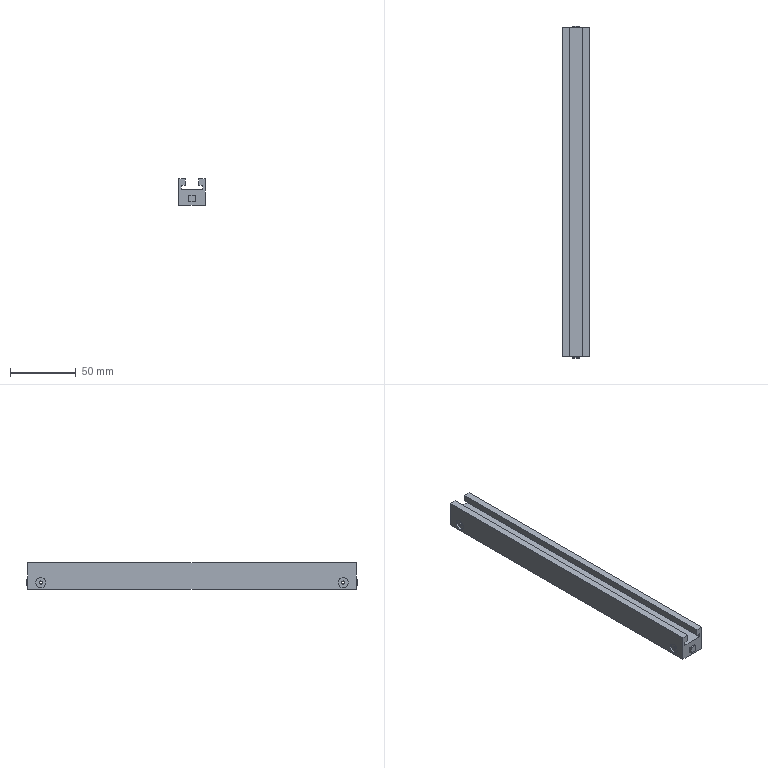Part | SolidWorks | features ICE 3, Extrusion 1, HoleWzd 1 | 1 solid | 38 faces | box 20 x 252.4 x 20 mm | volume 75264 mm3 | plane 26 | cylinder 8 | cone 4 | commonest cylinder face diameters 2.4 x4 7.619 x4
STEP:
#1=CARTESIAN_POINT('',(0.025,10.,-18.809));
#2=VERTEX_POINT('',#1);
#3=CARTESIAN_POINT('',(0.025,10.,-11.19));
#4=VERTEX_POINT('',#3);
#5=CARTESIAN_POINT('',(0.025,10.,-15.));
#6=DIRECTION('',(-1.,0.,0.));
#7=DIRECTION('',(0.,0.,1.));
#8=AXIS2_PLACEMENT_3D('',#5,#6,#7);
#9=CIRCLE('',#8,3.809);
#10=EDGE_CURVE('',#2,#4,#9,.T.);
#11=ORIENTED_EDGE('',*,*,#10,.F.);
#12=CARTESIAN_POINT('',(0.,10.,-18.834));
#13=VERTEX_POINT('',#12);
#14=CARTESIAN_POINT('',(0.,10.,-18.834));
#15=DIRECTION('',(-0.7071,0.,-0.7071));
#16=VECTOR('',#15,1000.);
#17=LINE('',#14,#16);
#18=EDGE_CURVE('',#2,#13,#17,.T.);
#19=ORIENTED_EDGE('',*,*,#18,.T.);
#20=CARTESIAN_POINT('',(0.,10.,-11.165));
#21=VERTEX_POINT('',#20);
#22=CARTESIAN_POINT('',(0.,10.,-15.));
#23=DIRECTION('',(-1.,0.,0.));
#24=DIRECTION('',(0.,0.,1.));
#25=AXIS2_PLACEMENT_3D('',#22,#23,#24);
#26=CIRCLE('',#25,3.835);
#27=EDGE_CURVE('',#13,#21,#26,.T.);
#28=ORIENTED_EDGE('',*,*,#27,.T.);
#29=CARTESIAN_POINT('',(0.,10.,-11.165));
#30=DIRECTION('',(-0.7071,0.,0.7071));
#31=VECTOR('',#30,1000.);
#32=LINE('',#29,#31);
#33=EDGE_CURVE('',#4,#21,#32,.T.);
#34=ORIENTED_EDGE('',*,*,#33,.F.);
#35=EDGE_LOOP('',(#11,#19,#28,#34));
#36=FACE_OUTER_BOUND('',#35,.T.);
#37=CARTESIAN_POINT('',(0.,10.,-15.));
#38=DIRECTION('',(-1.,0.,0.));
#39=DIRECTION('',(0.,0.,1.));
#40=AXIS2_PLACEMENT_3D('',#37,#38,#39);
#41=CONICAL_SURFACE('',#40,3.835,0.7854);
#42=ADVANCED_FACE('',(#36),#41,.F.);
#43=CARTESIAN_POINT('',(1.4,10.,-18.809));
#44=VERTEX_POINT('',#43);
#45=CARTESIAN_POINT('',(1.4,10.,-11.19));
#46=VERTEX_POINT('',#45);
#47=CARTESIAN_POINT('',(1.4,10.,-15.));
#48=DIRECTION('',(-1.,0.,0.));
#49=DIRECTION('',(0.,0.,1.));
#50=AXIS2_PLACEMENT_3D('',#47,#48,#49);
#51=CIRCLE('',#50,3.809);
#52=EDGE_CURVE('',#44,#46,#51,.T.);
#53=ORIENTED_EDGE('',*,*,#52,.F.);
#54=CARTESIAN_POINT('',(0.,10.,-18.809));
#55=DIRECTION('',(-1.,0.,0.));
#56=VECTOR('',#55,1000.);
#57=LINE('',#54,#56);
#58=EDGE_CURVE('',#44,#2,#57,.T.);
#59=ORIENTED_EDGE('',*,*,#58,.T.);
#60=ORIENTED_EDGE('',*,*,#10,.T.);
#61=CARTESIAN_POINT('',(0.,10.,-11.19));
#62=DIRECTION('',(-1.,0.,0.));
#63=VECTOR('',#62,1000.);
#64=LINE('',#61,#63);
#65=EDGE_CURVE('',#46,#4,#64,.T.);
#66=ORIENTED_EDGE('',*,*,#65,.F.);
#67=EDGE_LOOP('',(#53,#59,#60,#66));
#68=FACE_OUTER_BOUND('',#67,.T.);
#69=CARTESIAN_POINT('',(0.,10.,-15.));
#70=DIRECTION('',(-1.,0.,0.));
#71=DIRECTION('',(0.,0.,1.));
#72=AXIS2_PLACEMENT_3D('',#69,#70,#71);
#73=CYLINDRICAL_SURFACE('',#72,3.809);
#74=ADVANCED_FACE('',(#68),#73,.F.);
#75=CARTESIAN_POINT('',(20.,10.,-16.2));
#76=VERTEX_POINT('',#75);
#77=CARTESIAN_POINT('',(20.,10.,-13.8));
#78=VERTEX_POINT('',#77);
#79=CARTESIAN_POINT('',(20.,10.,-15.));
#80=DIRECTION('',(-1.,0.,0.));
#81=DIRECTION('',(0.,0.,1.));
#82=AXIS2_PLACEMENT_3D('',#79,#80,#81);
#83=CIRCLE('',#82,1.2);
#84=EDGE_CURVE('',#76,#78,#83,.T.);
#85=ORIENTED_EDGE('',*,*,#84,.F.);
#86=CARTESIAN_POINT('',(1.4,10.,-16.2));
#87=VERTEX_POINT('',#86);
#88=CARTESIAN_POINT('',(0.,10.,-16.2));
#89=DIRECTION('',(-1.,0.,0.));
#90=VECTOR('',#89,1000.);
#91=LINE('',#88,#90);
#92=EDGE_CURVE('',#76,#87,#91,.T.);
#93=ORIENTED_EDGE('',*,*,#92,.T.);
#94=CARTESIAN_POINT('',(1.4,10.,-13.8));
#95=VERTEX_POINT('',#94);
#96=CARTESIAN_POINT('',(1.4,10.,-15.));
#97=DIRECTION('',(-1.,0.,0.));
#98=DIRECTION('',(0.,0.,1.));
#99=AXIS2_PLACEMENT_3D('',#96,#97,#98);
#100=CIRCLE('',#99,1.2);
#101=EDGE_CURVE('',#87,#95,#100,.T.);
#102=ORIENTED_EDGE('',*,*,#101,.T.);
#103=CARTESIAN_POINT('',(0.,10.,-13.8));
#104=DIRECTION('',(-1.,0.,0.));
#105=VECTOR('',#104,1000.);
#106=LINE('',#103,#105);
#107=EDGE_CURVE('',#78,#95,#106,.T.);
#108=ORIENTED_EDGE('',*,*,#107,.F.);
#109=EDGE_LOOP('',(#85,#93,#102,#108));
#110=FACE_OUTER_BOUND('',#109,.T.);
#111=CARTESIAN_POINT('',(0.,10.,-15.));
#112=DIRECTION('',(-1.,0.,0.));
#113=DIRECTION('',(0.,0.,1.));
#114=AXIS2_PLACEMENT_3D('',#111,#112,#113);
#115=CYLINDRICAL_SURFACE('',#114,1.2);
#116=ADVANCED_FACE('',(#110),#115,.F.);
#117=CARTESIAN_POINT('',(0.025,240.,-18.809));
#118=VERTEX_POINT('',#117);
#119=CARTESIAN_POINT('',(0.025,240.,-11.191));
#120=VERTEX_POINT('',#119);
#121=CARTESIAN_POINT('',(0.025,240.,-15.));
#122=DIRECTION('',(-1.,0.,0.));
#123=DIRECTION('',(0.,0.,1.));
#124=AXIS2_PLACEMENT_3D('',#121,#122,#123);
#125=CIRCLE('',#124,3.809);
#126=EDGE_CURVE('',#118,#120,#125,.T.);
#127=ORIENTED_EDGE('',*,*,#126,.F.);
#128=CARTESIAN_POINT('',(0.,240.,-18.834));
#129=VERTEX_POINT('',#128);
#130=CARTESIAN_POINT('',(0.,240.,-18.834));
#131=DIRECTION('',(-0.7071,0.,-0.7071));
#132=VECTOR('',#131,1000.);
#133=LINE('',#130,#132);
#134=EDGE_CURVE('',#118,#129,#133,.T.);
#135=ORIENTED_EDGE('',*,*,#134,.T.);
#136=CARTESIAN_POINT('',(0.,240.,-11.166));
#137=VERTEX_POINT('',#136);
#138=CARTESIAN_POINT('',(0.,240.,-15.));
#139=DIRECTION('',(-1.,0.,0.));
#140=DIRECTION('',(0.,0.,1.));
#141=AXIS2_PLACEMENT_3D('',#138,#139,#140);
#142=CIRCLE('',#141,3.834);
#143=EDGE_CURVE('',#129,#137,#142,.T.);
#144=ORIENTED_EDGE('',*,*,#143,.T.);
#145=CARTESIAN_POINT('',(0.,240.,-11.166));
#146=DIRECTION('',(-0.7071,0.,0.7071));
#147=VECTOR('',#146,1000.);
#148=LINE('',#145,#147);
#149=EDGE_CURVE('',#120,#137,#148,.T.);
#150=ORIENTED_EDGE('',*,*,#149,.F.);
#151=EDGE_LOOP('',(#127,#135,#144,#150));
#152=FACE_OUTER_BOUND('',#151,.T.);
#153=CARTESIAN_POINT('',(0.,240.,-15.));
#154=DIRECTION('',(-1.,0.,0.));
#155=DIRECTION('',(0.,0.,1.));
#156=AXIS2_PLACEMENT_3D('',#153,#154,#155);
#157=CONICAL_SURFACE('',#156,3.834,0.7854);
#158=ADVANCED_FACE('',(#152),#157,.F.);
#159=CARTESIAN_POINT('',(1.4,240.,-18.809));
#160=VERTEX_POINT('',#159);
#161=CARTESIAN_POINT('',(1.4,240.,-11.191));
#162=VERTEX_POINT('',#161);
#163=CARTESIAN_POINT('',(1.4,240.,-15.));
#164=DIRECTION('',(-1.,0.,0.));
#165=DIRECTION('',(0.,0.,1.));
#166=AXIS2_PLACEMENT_3D('',#163,#164,#165);
#167=CIRCLE('',#166,3.809);
#168=EDGE_CURVE('',#160,#162,#167,.T.);
#169=ORIENTED_EDGE('',*,*,#168,.F.);
#170=CARTESIAN_POINT('',(0.,240.,-18.809));
#171=DIRECTION('',(-1.,0.,0.));
#172=VECTOR('',#171,1000.);
#173=LINE('',#170,#172);
#174=EDGE_CURVE('',#160,#118,#173,.T.);
#175=ORIENTED_EDGE('',*,*,#174,.T.);
#176=ORIENTED_EDGE('',*,*,#126,.T.);
#177=CARTESIAN_POINT('',(0.,240.,-11.191));
#178=DIRECTION('',(-1.,0.,0.));
#179=VECTOR('',#178,1000.);
#180=LINE('',#177,#179);
#181=EDGE_CURVE('',#162,#120,#180,.T.);
#182=ORIENTED_EDGE('',*,*,#181,.F.);
#183=EDGE_LOOP('',(#169,#175,#176,#182));
#184=FACE_OUTER_BOUND('',#183,.T.);
#185=CARTESIAN_POINT('',(0.,240.,-15.));
#186=DIRECTION('',(-1.,0.,0.));
#187=DIRECTION('',(0.,0.,1.));
#188=AXIS2_PLACEMENT_3D('',#185,#186,#187);
#189=CYLINDRICAL_SURFACE('',#188,3.809);
#190=ADVANCED_FACE('',(#184),#189,.F.);
#191=CARTESIAN_POINT('',(20.,240.,-16.2));
#192=VERTEX_POINT('',#191);
#193=CARTESIAN_POINT('',(20.,240.,-13.8));
#194=VERTEX_POINT('',#193);
#195=CARTESIAN_POINT('',(20.,240.,-15.));
#196=DIRECTION('',(-1.,0.,0.));
#197=DIRECTION('',(0.,0.,1.));
#198=AXIS2_PLACEMENT_3D('',#195,#196,#197);
#199=CIRCLE('',#198,1.2);
#200=EDGE_CURVE('',#192,#194,#199,.T.);
#201=ORIENTED_EDGE('',*,*,#200,.F.);
#202=CARTESIAN_POINT('',(1.4,240.,-16.2));
#203=VERTEX_POINT('',#202);
#204=CARTESIAN_POINT('',(0.,240.,-16.2));
#205=DIRECTION('',(-1.,0.,0.));
#206=VECTOR('',#205,1000.);
#207=LINE('',#204,#206);
#208=EDGE_CURVE('',#192,#203,#207,.T.);
#209=ORIENTED_EDGE('',*,*,#208,.T.);
#210=CARTESIAN_POINT('',(1.4,240.,-13.8));
#211=VERTEX_POINT('',#210);
#212=CARTESIAN_POINT('',(1.4,240.,-15.));
#213=DIRECTION('',(-1.,0.,0.));
#214=DIRECTION('',(0.,0.,1.));
#215=AXIS2_PLACEMENT_3D('',#212,#213,#214);
#216=CIRCLE('',#215,1.2);
#217=EDGE_CURVE('',#203,#211,#216,.T.);
#218=ORIENTED_EDGE('',*,*,#217,.T.);
#219=CARTESIAN_POINT('',(0.,240.,-13.8));
#220=DIRECTION('',(-1.,0.,0.));
#221=VECTOR('',#220,1000.);
#222=LINE('',#219,#221);
#223=EDGE_CURVE('',#194,#211,#222,.T.);
#224=ORIENTED_EDGE('',*,*,#223,.F.);
#225=EDGE_LOOP('',(#201,#209,#218,#224));
#226=FACE_OUTER_BOUND('',#225,.T.);
#227=CARTESIAN_POINT('',(0.,240.,-15.));
#228=DIRECTION('',(-1.,0.,0.));
#229=DIRECTION('',(0.,0.,1.));
#230=AXIS2_PLACEMENT_3D('',#227,#228,#229);
#231=CYLINDRICAL_SURFACE('',#230,1.2);
#232=ADVANCED_FACE('',(#226),#231,.F.);
#233=CARTESIAN_POINT('',(0.,0.,0.));
#234=VERTEX_POINT('',#233);
#235=CARTESIAN_POINT('',(5.,0.,0.));
#236=VERTEX_POINT('',#235);
#237=CARTESIAN_POINT('',(5.,0.,0.));
#238=DIRECTION('',(1.,0.,0.));
#239=VECTOR('',#238,1000.);
#240=LINE('',#237,#239);
#241=EDGE_CURVE('',#234,#236,#240,.T.);
#242=ORIENTED_EDGE('',*,*,#241,.F.);
#243=CARTESIAN_POINT('',(0.,0.,-20.));
#244=VERTEX_POINT('',#243);
#245=CARTESIAN_POINT('',(0.,0.,0.));
#246=DIRECTION('',(0.,0.,1.));
#247=VECTOR('',#246,1000.);
#248=LINE('',#245,#247);
#249=EDGE_CURVE('',#244,#234,#248,.T.);
#250=ORIENTED_EDGE('',*,*,#249,.F.);
#251=CARTESIAN_POINT('',(20.,0.,-20.));
#252=VERTEX_POINT('',#251);
#253=CARTESIAN_POINT('',(0.,0.,-20.));
#254=DIRECTION('',(-1.,0.,0.));
#255=VECTOR('',#254,1000.);
#256=LINE('',#253,#255);
#257=EDGE_CURVE('',#252,#244,#256,.T.);
#258=ORIENTED_EDGE('',*,*,#257,.F.);
#259=CARTESIAN_POINT('',(20.,0.,0.));
#260=VERTEX_POINT('',#259);
#261=CARTESIAN_POINT('',(20.,0.,-20.));
#262=DIRECTION('',(0.,0.,-1.));
#263=VECTOR('',#262,1000.);
#264=LINE('',#261,#263);
#265=EDGE_CURVE('',#260,#252,#264,.T.);
#266=ORIENTED_EDGE('',*,*,#265,.F.);
#267=CARTESIAN_POINT('',(15.,0.,0.));
#268=VERTEX_POINT('',#267);
#269=CARTESIAN_POINT('',(20.,0.,0.));
#270=DIRECTION('',(1.,0.,0.));
#271=VECTOR('',#270,1000.);
#272=LINE('',#269,#271);
#273=EDGE_CURVE('',#268,#260,#272,.T.);
#274=ORIENTED_EDGE('',*,*,#273,.F.);
#275=CARTESIAN_POINT('',(15.,0.,-5.));
#276=VERTEX_POINT('',#275);
#277=CARTESIAN_POINT('',(15.,0.,0.));
#278=DIRECTION('',(0.,0.,1.));
#279=VECTOR('',#278,1000.);
#280=LINE('',#277,#279);
#281=EDGE_CURVE('',#276,#268,#280,.T.);
#282=ORIENTED_EDGE('',*,*,#281,.F.);
#283=CARTESIAN_POINT('',(18.,0.,-5.));
#284=VERTEX_POINT('',#283);
#285=CARTESIAN_POINT('',(15.,0.,-5.));
#286=DIRECTION('',(-1.,0.,0.));
#287=VECTOR('',#286,1000.);
#288=LINE('',#285,#287);
#289=EDGE_CURVE('',#284,#276,#288,.T.);
#290=ORIENTED_EDGE('',*,*,#289,.F.);
#291=CARTESIAN_POINT('',(18.,0.,-8.));
#292=VERTEX_POINT('',#291);
#293=CARTESIAN_POINT('',(18.,0.,-5.));
#294=DIRECTION('',(0.,0.,1.));
#295=VECTOR('',#294,1000.);
#296=LINE('',#293,#295);
#297=EDGE_CURVE('',#292,#284,#296,.T.);
#298=ORIENTED_EDGE('',*,*,#297,.F.);
#299=CARTESIAN_POINT('',(2.,0.,-8.));
#300=VERTEX_POINT('',#299);
#301=CARTESIAN_POINT('',(2.,0.,-8.));
#302=DIRECTION('',(1.,0.,0.));
#303=VECTOR('',#302,1000.);
#304=LINE('',#301,#303);
#305=EDGE_CURVE('',#300,#292,#304,.T.);
#306=ORIENTED_EDGE('',*,*,#305,.F.);
#307=CARTESIAN_POINT('',(2.,0.,-5.));
#308=VERTEX_POINT('',#307);
#309=CARTESIAN_POINT('',(2.,0.,-8.));
#310=DIRECTION('',(0.,0.,-1.));
#311=VECTOR('',#310,1000.);
#312=LINE('',#309,#311);
#313=EDGE_CURVE('',#308,#300,#312,.T.);
#314=ORIENTED_EDGE('',*,*,#313,.F.);
#315=CARTESIAN_POINT('',(5.,0.,-5.));
#316=VERTEX_POINT('',#315);
#317=CARTESIAN_POINT('',(2.,0.,-5.));
#318=DIRECTION('',(-1.,0.,0.));
#319=VECTOR('',#318,1000.);
#320=LINE('',#317,#319);
#321=EDGE_CURVE('',#316,#308,#320,.T.);
#322=ORIENTED_EDGE('',*,*,#321,.F.);
#323=CARTESIAN_POINT('',(5.,0.,-5.));
#324=DIRECTION('',(0.,0.,-1.));
#325=VECTOR('',#324,1000.);
#326=LINE('',#323,#325);
#327=EDGE_CURVE('',#236,#316,#326,.T.);
#328=ORIENTED_EDGE('',*,*,#327,.F.);
#329=EDGE_LOOP('',(#242,#250,#258,#266,#274,#282,#290,#298,#306,#314,#322,#328));
#330=FACE_OUTER_BOUND('',#329,.T.);
#331=CARTESIAN_POINT('',(12.5,0.,-17.5));
#332=VERTEX_POINT('',#331);
#333=CARTESIAN_POINT('',(7.5,0.,-17.5));
#334=VERTEX_POINT('',#333);
#335=CARTESIAN_POINT('',(0.,0.,-17.5));
#336=DIRECTION('',(-1.,0.,0.));
#337=VECTOR('',#336,1000.);
#338=LINE('',#335,#337);
#339=EDGE_CURVE('',#332,#334,#338,.T.);
#340=ORIENTED_EDGE('',*,*,#339,.T.);
#341=CARTESIAN_POINT('',(7.5,0.,-12.5));
#342=VERTEX_POINT('',#341);
#343=CARTESIAN_POINT('',(7.5,0.,0.));
#344=DIRECTION('',(0.,0.,1.));
#345=VECTOR('',#344,1000.);
#346=LINE('',#343,#345);
#347=EDGE_CURVE('',#334,#342,#346,.T.);
#348=ORIENTED_EDGE('',*,*,#347,.T.);
#349=CARTESIAN_POINT('',(12.5,0.,-12.5));
#350=VERTEX_POINT('',#349);
#351=CARTESIAN_POINT('',(0.,0.,-12.5));
#352=DIRECTION('',(-1.,0.,0.));
#353=VECTOR('',#352,1000.);
#354=LINE('',#351,#353);
#355=EDGE_CURVE('',#350,#342,#354,.T.);
#356=ORIENTED_EDGE('',*,*,#355,.F.);
#357=CARTESIAN_POINT('',(12.5,0.,0.));
#358=DIRECTION('',(0.,0.,1.));
#359=VECTOR('',#358,1000.);
#360=LINE('',#357,#359);
#361=EDGE_CURVE('',#332,#350,#360,.T.);
#362=ORIENTED_EDGE('',*,*,#361,.F.);
#363=EDGE_LOOP('',(#340,#348,#356,#362));
#364=FACE_BOUND('',#363,.T.);
#365=CARTESIAN_POINT('',(0.,0.,0.));
#366=DIRECTION('',(0.,-1.,0.));
#367=DIRECTION('',(0.,0.,-1.));
#368=AXIS2_PLACEMENT_3D('',#365,#366,#367);
#369=PLANE('',#368);
#370=ADVANCED_FACE('',(#330,#364),#369,.T.);
#371=CARTESIAN_POINT('',(0.,250.,0.));
#372=VERTEX_POINT('',#371);
#373=CARTESIAN_POINT('',(5.,250.,0.));
#374=VERTEX_POINT('',#373);
#375=CARTESIAN_POINT('',(5.,250.,0.));
#376=DIRECTION('',(1.,0.,0.));
#377=VECTOR('',#376,1000.);
#378=LINE('',#375,#377);
#379=EDGE_CURVE('',#372,#374,#378,.T.);
#380=ORIENTED_EDGE('',*,*,#379,.T.);
#381=CARTESIAN_POINT('',(5.,250.,-5.));
#382=VERTEX_POINT('',#381);
#383=CARTESIAN_POINT('',(5.,250.,-5.));
#384=DIRECTION('',(0.,0.,-1.));
#385=VECTOR('',#384,1000.);
#386=LINE('',#383,#385);
#387=EDGE_CURVE('',#374,#382,#386,.T.);
#388=ORIENTED_EDGE('',*,*,#387,.T.);
#389=CARTESIAN_POINT('',(2.,250.,-5.));
#390=VERTEX_POINT('',#389);
#391=CARTESIAN_POINT('',(2.,250.,-5.));
#392=DIRECTION('',(-1.,0.,0.));
#393=VECTOR('',#392,1000.);
#394=LINE('',#391,#393);
#395=EDGE_CURVE('',#382,#390,#394,.T.);
#396=ORIENTED_EDGE('',*,*,#395,.T.);
#397=CARTESIAN_POINT('',(2.,250.,-8.));
#398=VERTEX_POINT('',#397);
#399=CARTESIAN_POINT('',(2.,250.,-8.));
#400=DIRECTION('',(0.,0.,-1.));
#401=VECTOR('',#400,1000.);
#402=LINE('',#399,#401);
#403=EDGE_CURVE('',#390,#398,#402,.T.);
#404=ORIENTED_EDGE('',*,*,#403,.T.);
#405=CARTESIAN_POINT('',(18.,250.,-8.));
#406=VERTEX_POINT('',#405);
#407=CARTESIAN_POINT('',(2.,250.,-8.));
#408=DIRECTION('',(1.,0.,0.));
#409=VECTOR('',#408,1000.);
#410=LINE('',#407,#409);
#411=EDGE_CURVE('',#398,#406,#410,.T.);
#412=ORIENTED_EDGE('',*,*,#411,.T.);
#413=CARTESIAN_POINT('',(18.,250.,-5.));
#414=VERTEX_POINT('',#413);
#415=CARTESIAN_POINT('',(18.,250.,-5.));
#416=DIRECTION('',(0.,0.,1.));
#417=VECTOR('',#416,1000.);
#418=LINE('',#415,#417);
#419=EDGE_CURVE('',#406,#414,#418,.T.);
#420=ORIENTED_EDGE('',*,*,#419,.T.);
#421=CARTESIAN_POINT('',(15.,250.,-5.));
#422=VERTEX_POINT('',#421);
#423=CARTESIAN_POINT('',(15.,250.,-5.));
#424=DIRECTION('',(-1.,0.,0.));
#425=VECTOR('',#424,1000.);
#426=LINE('',#423,#425);
#427=EDGE_CURVE('',#414,#422,#426,.T.);
#428=ORIENTED_EDGE('',*,*,#427,.T.);
#429=CARTESIAN_POINT('',(15.,250.,0.));
#430=VERTEX_POINT('',#429);
#431=CARTESIAN_POINT('',(15.,250.,0.));
#432=DIRECTION('',(0.,0.,1.));
#433=VECTOR('',#432,1000.);
#434=LINE('',#431,#433);
#435=EDGE_CURVE('',#422,#430,#434,.T.);
#436=ORIENTED_EDGE('',*,*,#435,.T.);
#437=CARTESIAN_POINT('',(20.,250.,0.));
#438=VERTEX_POINT('',#437);
#439=CARTESIAN_POINT('',(20.,250.,0.));
#440=DIRECTION('',(1.,0.,0.));
#441=VECTOR('',#440,1000.);
#442=LINE('',#439,#441);
#443=EDGE_CURVE('',#430,#438,#442,.T.);
#444=ORIENTED_EDGE('',*,*,#443,.T.);
#445=CARTESIAN_POINT('',(20.,250.,-20.));
#446=VERTEX_POINT('',#445);
#447=CARTESIAN_POINT('',(20.,250.,-20.));
#448=DIRECTION('',(0.,0.,-1.));
#449=VECTOR('',#448,1000.);
#450=LINE('',#447,#449);
#451=EDGE_CURVE('',#438,#446,#450,.T.);
#452=ORIENTED_EDGE('',*,*,#451,.T.);
#453=CARTESIAN_POINT('',(0.,250.,-20.));
#454=VERTEX_POINT('',#453);
#455=CARTESIAN_POINT('',(0.,250.,-20.));
#456=DIRECTION('',(-1.,0.,0.));
#457=VECTOR('',#456,1000.);
#458=LINE('',#455,#457);
#459=EDGE_CURVE('',#446,#454,#458,.T.);
#460=ORIENTED_EDGE('',*,*,#459,.T.);
#461=CARTESIAN_POINT('',(0.,250.,0.));
#462=DIRECTION('',(0.,0.,1.));
#463=VECTOR('',#462,1000.);
#464=LINE('',#461,#463);
#465=EDGE_CURVE('',#454,#372,#464,.T.);
#466=ORIENTED_EDGE('',*,*,#465,.T.);
#467=EDGE_LOOP('',(#380,#388,#396,#404,#412,#420,#428,#436,#444,#452,#460,#466));
#468=FACE_OUTER_BOUND('',#467,.T.);
#469=CARTESIAN_POINT('',(7.5,250.,-12.5));
#470=VERTEX_POINT('',#469);
#471=CARTESIAN_POINT('',(12.5,250.,-12.5));
#472=VERTEX_POINT('',#471);
#473=CARTESIAN_POINT('',(0.,250.,-12.5));
#474=DIRECTION('',(1.,0.,0.));
#475=VECTOR('',#474,1000.);
#476=LINE('',#473,#475);
#477=EDGE_CURVE('',#470,#472,#476,.T.);
#478=ORIENTED_EDGE('',*,*,#477,.F.);
#479=CARTESIAN_POINT('',(7.5,250.,-17.5));
#480=VERTEX_POINT('',#479);
#481=CARTESIAN_POINT('',(7.5,250.,0.));
#482=DIRECTION('',(0.,0.,-1.));
#483=VECTOR('',#482,1000.);
#484=LINE('',#481,#483);
#485=EDGE_CURVE('',#470,#480,#484,.T.);
#486=ORIENTED_EDGE('',*,*,#485,.T.);
#487=CARTESIAN_POINT('',(12.5,250.,-17.5));
#488=VERTEX_POINT('',#487);
#489=CARTESIAN_POINT('',(0.,250.,-17.5));
#490=DIRECTION('',(1.,0.,0.));
#491=VECTOR('',#490,1000.);
#492=LINE('',#489,#491);
#493=EDGE_CURVE('',#480,#488,#492,.T.);
#494=ORIENTED_EDGE('',*,*,#493,.T.);
#495=CARTESIAN_POINT('',(12.5,250.,0.));
#496=DIRECTION('',(0.,0.,-1.));
#497=VECTOR('',#496,1000.);
#498=LINE('',#495,#497);
#499=EDGE_CURVE('',#472,#488,#498,.T.);
#500=ORIENTED_EDGE('',*,*,#499,.F.);
#501=EDGE_LOOP('',(#478,#486,#494,#500));
#502=FACE_BOUND('',#501,.T.);
#503=CARTESIAN_POINT('',(0.,250.,0.));
#504=DIRECTION('',(0.,-1.,0.));
#505=DIRECTION('',(0.,0.,-1.));
#506=AXIS2_PLACEMENT_3D('',#503,#504,#505);
#507=PLANE('',#506);
#508=ADVANCED_FACE('',(#468,#502),#507,.F.);
#509=ORIENTED_EDGE('',*,*,#241,.T.);
#510=CARTESIAN_POINT('',(5.,250.,0.));
#511=DIRECTION('',(0.,-1.,0.));
#512=VECTOR('',#511,1000.);
#513=LINE('',#510,#512);
#514=EDGE_CURVE('',#374,#236,#513,.T.);
#515=ORIENTED_EDGE('',*,*,#514,.F.);
#516=ORIENTED_EDGE('',*,*,#379,.F.);
#517=CARTESIAN_POINT('',(0.,250.,0.));
#518=DIRECTION('',(0.,-1.,0.));
#519=VECTOR('',#518,1000.);
#520=LINE('',#517,#519);
#521=EDGE_CURVE('',#372,#234,#520,.T.);
#522=ORIENTED_EDGE('',*,*,#521,.T.);
#523=EDGE_LOOP('',(#509,#515,#516,#522));
#524=FACE_OUTER_BOUND('',#523,.T.);
#525=CARTESIAN_POINT('',(5.,250.,0.));
#526=DIRECTION('',(0.,0.,-1.));
#527=DIRECTION('',(-1.,0.,0.));
#528=AXIS2_PLACEMENT_3D('',#525,#526,#527);
#529=PLANE('',#528);
#530=ADVANCED_FACE('',(#524),#529,.F.);
#531=ORIENTED_EDGE('',*,*,#327,.T.);
#532=CARTESIAN_POINT('',(5.,250.,-5.));
#533=DIRECTION('',(0.,-1.,0.));
#534=VECTOR('',#533,1000.);
#535=LINE('',#532,#534);
#536=EDGE_CURVE('',#382,#316,#535,.T.);
#537=ORIENTED_EDGE('',*,*,#536,.F.);
#538=ORIENTED_EDGE('',*,*,#387,.F.);
#539=ORIENTED_EDGE('',*,*,#514,.T.);
#540=EDGE_LOOP('',(#531,#537,#538,#539));
#541=FACE_OUTER_BOUND('',#540,.T.);
#542=CARTESIAN_POINT('',(5.,250.,-5.));
#543=DIRECTION('',(-1.,0.,0.));
#544=DIRECTION('',(0.,0.,1.));
#545=AXIS2_PLACEMENT_3D('',#542,#543,#544);
#546=PLANE('',#545);
#547=ADVANCED_FACE('',(#541),#546,.F.);
#548=ORIENTED_EDGE('',*,*,#321,.T.);
#549=CARTESIAN_POINT('',(2.,250.,-5.));
#550=DIRECTION('',(0.,-1.,0.));
#551=VECTOR('',#550,1000.);
#552=LINE('',#549,#551);
#553=EDGE_CURVE('',#390,#308,#552,.T.);
#554=ORIENTED_EDGE('',*,*,#553,.F.);
#555=ORIENTED_EDGE('',*,*,#395,.F.);
#556=ORIENTED_EDGE('',*,*,#536,.T.);
#557=EDGE_LOOP('',(#548,#554,#555,#556));
#558=FACE_OUTER_BOUND('',#557,.T.);
#559=CARTESIAN_POINT('',(2.,250.,-5.));
#560=DIRECTION('',(0.,0.,1.));
#561=DIRECTION('',(1.,0.,0.));
#562=AXIS2_PLACEMENT_3D('',#559,#560,#561);
#563=PLANE('',#562);
#564=ADVANCED_FACE('',(#558),#563,.F.);
#565=ORIENTED_EDGE('',*,*,#313,.T.);
#566=CARTESIAN_POINT('',(2.,250.,-8.));
#567=DIRECTION('',(0.,-1.,0.));
#568=VECTOR('',#567,1000.);
#569=LINE('',#566,#568);
#570=EDGE_CURVE('',#398,#300,#569,.T.);
#571=ORIENTED_EDGE('',*,*,#570,.F.);
#572=ORIENTED_EDGE('',*,*,#403,.F.);
#573=ORIENTED_EDGE('',*,*,#553,.T.);
#574=EDGE_LOOP('',(#565,#571,#572,#573));
#575=FACE_OUTER_BOUND('',#574,.T.);
#576=CARTESIAN_POINT('',(2.,250.,-8.));
#577=DIRECTION('',(-1.,0.,0.));
#578=DIRECTION('',(0.,0.,1.));
#579=AXIS2_PLACEMENT_3D('',#576,#577,#578);
#580=PLANE('',#579);
#581=ADVANCED_FACE('',(#575),#580,.F.);
#582=ORIENTED_EDGE('',*,*,#305,.T.);
#583=CARTESIAN_POINT('',(18.,250.,-8.));
#584=DIRECTION('',(0.,-1.,0.));
#585=VECTOR('',#584,1000.);
#586=LINE('',#583,#585);
#587=EDGE_CURVE('',#406,#292,#586,.T.);
#588=ORIENTED_EDGE('',*,*,#587,.F.);
#589=ORIENTED_EDGE('',*,*,#411,.F.);
#590=ORIENTED_EDGE('',*,*,#570,.T.);
#591=EDGE_LOOP('',(#582,#588,#589,#590));
#592=FACE_OUTER_BOUND('',#591,.T.);
#593=CARTESIAN_POINT('',(2.,250.,-8.));
#594=DIRECTION('',(0.,0.,-1.));
#595=DIRECTION('',(-1.,0.,0.));
#596=AXIS2_PLACEMENT_3D('',#593,#594,#595);
#597=PLANE('',#596);
#598=ADVANCED_FACE('',(#592),#597,.F.);
#599=ORIENTED_EDGE('',*,*,#297,.T.);
#600=CARTESIAN_POINT('',(18.,250.,-5.));
#601=DIRECTION('',(0.,-1.,0.));
#602=VECTOR('',#601,1000.);
#603=LINE('',#600,#602);
#604=EDGE_CURVE('',#414,#284,#603,.T.);
#605=ORIENTED_EDGE('',*,*,#604,.F.);
#606=ORIENTED_EDGE('',*,*,#419,.F.);
#607=ORIENTED_EDGE('',*,*,#587,.T.);
#608=EDGE_LOOP('',(#599,#605,#606,#607));
#609=FACE_OUTER_BOUND('',#608,.T.);
#610=CARTESIAN_POINT('',(18.,250.,-5.));
#611=DIRECTION('',(1.,0.,0.));
#612=DIRECTION('',(0.,0.,-1.));
#613=AXIS2_PLACEMENT_3D('',#610,#611,#612);
#614=PLANE('',#613);
#615=ADVANCED_FACE('',(#609),#614,.F.);
#616=ORIENTED_EDGE('',*,*,#289,.T.);
#617=CARTESIAN_POINT('',(15.,250.,-5.));
#618=DIRECTION('',(0.,-1.,0.));
#619=VECTOR('',#618,1000.);
#620=LINE('',#617,#619);
#621=EDGE_CURVE('',#422,#276,#620,.T.);
#622=ORIENTED_EDGE('',*,*,#621,.F.);
#623=ORIENTED_EDGE('',*,*,#427,.F.);
#624=ORIENTED_EDGE('',*,*,#604,.T.);
#625=EDGE_LOOP('',(#616,#622,#623,#624));
#626=FACE_OUTER_BOUND('',#625,.T.);
#627=CARTESIAN_POINT('',(15.,250.,-5.));
#628=DIRECTION('',(0.,0.,1.));
#629=DIRECTION('',(1.,0.,0.));
#630=AXIS2_PLACEMENT_3D('',#627,#628,#629);
#631=PLANE('',#630);
#632=ADVANCED_FACE('',(#626),#631,.F.);
#633=ORIENTED_EDGE('',*,*,#281,.T.);
#634=CARTESIAN_POINT('',(15.,250.,0.));
#635=DIRECTION('',(0.,-1.,0.));
#636=VECTOR('',#635,1000.);
#637=LINE('',#634,#636);
#638=EDGE_CURVE('',#430,#268,#637,.T.);
#639=ORIENTED_EDGE('',*,*,#638,.F.);
#640=ORIENTED_EDGE('',*,*,#435,.F.);
#641=ORIENTED_EDGE('',*,*,#621,.T.);
#642=EDGE_LOOP('',(#633,#639,#640,#641));
#643=FACE_OUTER_BOUND('',#642,.T.);
#644=CARTESIAN_POINT('',(15.,250.,0.));
#645=DIRECTION('',(1.,0.,0.));
#646=DIRECTION('',(0.,0.,-1.));
#647=AXIS2_PLACEMENT_3D('',#644,#645,#646);
#648=PLANE('',#647);
#649=ADVANCED_FACE('',(#643),#648,.F.);
#650=ORIENTED_EDGE('',*,*,#273,.T.);
#651=CARTESIAN_POINT('',(20.,250.,0.));
#652=DIRECTION('',(0.,-1.,0.));
#653=VECTOR('',#652,1000.);
#654=LINE('',#651,#653);
#655=EDGE_CURVE('',#438,#260,#654,.T.);
#656=ORIENTED_EDGE('',*,*,#655,.F.);
#657=ORIENTED_EDGE('',*,*,#443,.F.);
#658=ORIENTED_EDGE('',*,*,#638,.T.);
#659=EDGE_LOOP('',(#650,#656,#657,#658));
#660=FACE_OUTER_BOUND('',#659,.T.);
#661=CARTESIAN_POINT('',(20.,250.,0.));
#662=DIRECTION('',(0.,0.,-1.));
#663=DIRECTION('',(-1.,0.,0.));
#664=AXIS2_PLACEMENT_3D('',#661,#662,#663);
#665=PLANE('',#664);
#666=ADVANCED_FACE('',(#660),#665,.F.);
#667=CARTESIAN_POINT('',(20.,10.,-15.));
#668=DIRECTION('',(-1.,0.,0.));
#669=DIRECTION('',(0.,0.,1.));
#670=AXIS2_PLACEMENT_3D('',#667,#668,#669);
#671=CIRCLE('',#670,1.2);
#672=EDGE_CURVE('',#78,#76,#671,.T.);
#673=ORIENTED_EDGE('',*,*,#672,.T.);
#674=ORIENTED_EDGE('',*,*,#84,.T.);
#675=EDGE_LOOP('',(#673,#674));
#676=FACE_BOUND('',#675,.T.);
#677=CARTESIAN_POINT('',(20.,240.,-15.));
#678=DIRECTION('',(-1.,0.,0.));
#679=DIRECTION('',(0.,0.,1.));
#680=AXIS2_PLACEMENT_3D('',#677,#678,#679);
#681=CIRCLE('',#680,1.2);
#682=EDGE_CURVE('',#194,#192,#681,.T.);
#683=ORIENTED_EDGE('',*,*,#682,.T.);
#684=ORIENTED_EDGE('',*,*,#200,.T.);
#685=EDGE_LOOP('',(#683,#684));
#686=FACE_BOUND('',#685,.T.);
#687=ORIENTED_EDGE('',*,*,#265,.T.);
#688=CARTESIAN_POINT('',(20.,250.,-20.));
#689=DIRECTION('',(0.,-1.,0.));
#690=VECTOR('',#689,1000.);
#691=LINE('',#688,#690);
#692=EDGE_CURVE('',#446,#252,#691,.T.);
#693=ORIENTED_EDGE('',*,*,#692,.F.);
#694=ORIENTED_EDGE('',*,*,#451,.F.);
#695=ORIENTED_EDGE('',*,*,#655,.T.);
#696=EDGE_LOOP('',(#687,#693,#694,#695));
#697=FACE_OUTER_BOUND('',#696,.T.);
#698=CARTESIAN_POINT('',(20.,250.,-20.));
#699=DIRECTION('',(-1.,0.,0.));
#700=DIRECTION('',(0.,0.,1.));
#701=AXIS2_PLACEMENT_3D('',#698,#699,#700);
#702=PLANE('',#701);
#703=ADVANCED_FACE('',(#676,#686,#697),#702,.F.);
#704=ORIENTED_EDGE('',*,*,#257,.T.);
#705=CARTESIAN_POINT('',(0.,250.,-20.));
#706=DIRECTION('',(0.,-1.,0.));
#707=VECTOR('',#706,1000.);
#708=LINE('',#705,#707);
#709=EDGE_CURVE('',#454,#244,#708,.T.);
#710=ORIENTED_EDGE('',*,*,#709,.F.);
#711=ORIENTED_EDGE('',*,*,#459,.F.);
#712=ORIENTED_EDGE('',*,*,#692,.T.);
#713=EDGE_LOOP('',(#704,#710,#711,#712));
#714=FACE_OUTER_BOUND('',#713,.T.);
#715=CARTESIAN_POINT('',(0.,250.,-20.));
#716=DIRECTION('',(0.,0.,1.));
#717=DIRECTION('',(1.,0.,0.));
#718=AXIS2_PLACEMENT_3D('',#715,#716,#717);
#719=PLANE('',#718);
#720=ADVANCED_FACE('',(#714),#719,.F.);
#721=CARTESIAN_POINT('',(0.,10.,-15.));
#722=DIRECTION('',(-1.,0.,0.));
#723=DIRECTION('',(0.,0.,1.));
#724=AXIS2_PLACEMENT_3D('',#721,#722,#723);
#725=CIRCLE('',#724,3.835);
#726=EDGE_CURVE('',#21,#13,#725,.T.);
#727=ORIENTED_EDGE('',*,*,#726,.F.);
#728=ORIENTED_EDGE('',*,*,#27,.F.);
#729=EDGE_LOOP('',(#727,#728));
#730=FACE_BOUND('',#729,.T.);
#731=CARTESIAN_POINT('',(0.,240.,-15.));
#732=DIRECTION('',(-1.,0.,0.));
#733=DIRECTION('',(0.,0.,1.));
#734=AXIS2_PLACEMENT_3D('',#731,#732,#733);
#735=CIRCLE('',#734,3.834);
#736=EDGE_CURVE('',#137,#129,#735,.T.);
#737=ORIENTED_EDGE('',*,*,#736,.F.);
#738=ORIENTED_EDGE('',*,*,#143,.F.);
#739=EDGE_LOOP('',(#737,#738));
#740=FACE_BOUND('',#739,.T.);
#741=ORIENTED_EDGE('',*,*,#249,.T.);
#742=ORIENTED_EDGE('',*,*,#521,.F.);
#743=ORIENTED_EDGE('',*,*,#465,.F.);
#744=ORIENTED_EDGE('',*,*,#709,.T.);
#745=EDGE_LOOP('',(#741,#742,#743,#744));
#746=FACE_OUTER_BOUND('',#745,.T.);
#747=CARTESIAN_POINT('',(0.,250.,0.));
#748=DIRECTION('',(1.,0.,0.));
#749=DIRECTION('',(0.,0.,-1.));
#750=AXIS2_PLACEMENT_3D('',#747,#748,#749);
#751=PLANE('',#750);
#752=ADVANCED_FACE('',(#730,#740,#746),#751,.F.);
#753=ORIENTED_EDGE('',*,*,#208,.F.);
#754=ORIENTED_EDGE('',*,*,#682,.F.);
#755=ORIENTED_EDGE('',*,*,#223,.T.);
#756=CARTESIAN_POINT('',(1.4,240.,-15.));
#757=DIRECTION('',(-1.,0.,0.));
#758=DIRECTION('',(0.,0.,1.));
#759=AXIS2_PLACEMENT_3D('',#756,#757,#758);
#760=CIRCLE('',#759,1.2);
#761=EDGE_CURVE('',#211,#203,#760,.T.);
#762=ORIENTED_EDGE('',*,*,#761,.T.);
#763=EDGE_LOOP('',(#753,#754,#755,#762));
#764=FACE_OUTER_BOUND('',#763,.T.);
#765=CARTESIAN_POINT('',(0.,240.,-15.));
#766=DIRECTION('',(-1.,0.,0.));
#767=DIRECTION('',(0.,0.,1.));
#768=AXIS2_PLACEMENT_3D('',#765,#766,#767);
#769=CYLINDRICAL_SURFACE('',#768,1.2);
#770=ADVANCED_FACE('',(#764),#769,.F.);
#771=ORIENTED_EDGE('',*,*,#761,.F.);
#772=ORIENTED_EDGE('',*,*,#217,.F.);
#773=EDGE_LOOP('',(#771,#772));
#774=FACE_BOUND('',#773,.T.);
#775=CARTESIAN_POINT('',(1.4,240.,-15.));
#776=DIRECTION('',(-1.,0.,0.));
#777=DIRECTION('',(0.,0.,1.));
#778=AXIS2_PLACEMENT_3D('',#775,#776,#777);
#779=CIRCLE('',#778,3.809);
#780=EDGE_CURVE('',#162,#160,#779,.T.);
#781=ORIENTED_EDGE('',*,*,#780,.T.);
#782=ORIENTED_EDGE('',*,*,#168,.T.);
#783=EDGE_LOOP('',(#781,#782));
#784=FACE_OUTER_BOUND('',#783,.T.);
#785=CARTESIAN_POINT('',(1.4,241.2,-15.));
#786=DIRECTION('',(1.,0.,0.));
#787=DIRECTION('',(0.,0.,-1.));
#788=AXIS2_PLACEMENT_3D('',#785,#786,#787);
#789=PLANE('',#788);
#790=ADVANCED_FACE('',(#774,#784),#789,.F.);
#791=ORIENTED_EDGE('',*,*,#174,.F.);
#792=ORIENTED_EDGE('',*,*,#780,.F.);
#793=ORIENTED_EDGE('',*,*,#181,.T.);
#794=CARTESIAN_POINT('',(0.025,240.,-15.));
#795=DIRECTION('',(-1.,0.,0.));
#796=DIRECTION('',(0.,0.,1.));
#797=AXIS2_PLACEMENT_3D('',#794,#795,#796);
#798=CIRCLE('',#797,3.809);
#799=EDGE_CURVE('',#120,#118,#798,.T.);
#800=ORIENTED_EDGE('',*,*,#799,.T.);
#801=EDGE_LOOP('',(#791,#792,#793,#800));
#802=FACE_OUTER_BOUND('',#801,.T.);
#803=CARTESIAN_POINT('',(0.,240.,-15.));
#804=DIRECTION('',(-1.,0.,0.));
#805=DIRECTION('',(0.,0.,1.));
#806=AXIS2_PLACEMENT_3D('',#803,#804,#805);
#807=CYLINDRICAL_SURFACE('',#806,3.809);
#808=ADVANCED_FACE('',(#802),#807,.F.);
#809=ORIENTED_EDGE('',*,*,#134,.F.);
#810=ORIENTED_EDGE('',*,*,#799,.F.);
#811=ORIENTED_EDGE('',*,*,#149,.T.);
#812=ORIENTED_EDGE('',*,*,#736,.T.);
#813=EDGE_LOOP('',(#809,#810,#811,#812));
#814=FACE_OUTER_BOUND('',#813,.T.);
#815=CARTESIAN_POINT('',(0.,240.,-15.));
#816=DIRECTION('',(-1.,0.,0.));
#817=DIRECTION('',(0.,0.,1.));
#818=AXIS2_PLACEMENT_3D('',#815,#816,#817);
#819=CONICAL_SURFACE('',#818,3.834,0.7854);
#820=ADVANCED_FACE('',(#814),#819,.F.);
#821=ORIENTED_EDGE('',*,*,#92,.F.);
#822=ORIENTED_EDGE('',*,*,#672,.F.);
#823=ORIENTED_EDGE('',*,*,#107,.T.);
#824=CARTESIAN_POINT('',(1.4,10.,-15.));
#825=DIRECTION('',(-1.,0.,0.));
#826=DIRECTION('',(0.,0.,1.));
#827=AXIS2_PLACEMENT_3D('',#824,#825,#826);
#828=CIRCLE('',#827,1.2);
#829=EDGE_CURVE('',#95,#87,#828,.T.);
#830=ORIENTED_EDGE('',*,*,#829,.T.);
#831=EDGE_LOOP('',(#821,#822,#823,#830));
#832=FACE_OUTER_BOUND('',#831,.T.);
#833=CARTESIAN_POINT('',(0.,10.,-15.));
#834=DIRECTION('',(-1.,0.,0.));
#835=DIRECTION('',(0.,0.,1.));
#836=AXIS2_PLACEMENT_3D('',#833,#834,#835);
#837=CYLINDRICAL_SURFACE('',#836,1.2);
#838=ADVANCED_FACE('',(#832),#837,.F.);
#839=ORIENTED_EDGE('',*,*,#829,.F.);
#840=ORIENTED_EDGE('',*,*,#101,.F.);
#841=EDGE_LOOP('',(#839,#840));
#842=FACE_BOUND('',#841,.T.);
#843=CARTESIAN_POINT('',(1.4,10.,-15.));
#844=DIRECTION('',(-1.,0.,0.));
#845=DIRECTION('',(0.,0.,1.));
#846=AXIS2_PLACEMENT_3D('',#843,#844,#845);
#847=CIRCLE('',#846,3.809);
#848=EDGE_CURVE('',#46,#44,#847,.T.);
#849=ORIENTED_EDGE('',*,*,#848,.T.);
#850=ORIENTED_EDGE('',*,*,#52,.T.);
#851=EDGE_LOOP('',(#849,#850));
#852=FACE_OUTER_BOUND('',#851,.T.);
#853=CARTESIAN_POINT('',(1.4,11.2,-15.));
#854=DIRECTION('',(1.,0.,0.));
#855=DIRECTION('',(0.,0.,-1.));
#856=AXIS2_PLACEMENT_3D('',#853,#854,#855);
#857=PLANE('',#856);
#858=ADVANCED_FACE('',(#842,#852),#857,.F.);
#859=ORIENTED_EDGE('',*,*,#58,.F.);
#860=ORIENTED_EDGE('',*,*,#848,.F.);
#861=ORIENTED_EDGE('',*,*,#65,.T.);
#862=CARTESIAN_POINT('',(0.025,10.,-15.));
#863=DIRECTION('',(-1.,0.,0.));
#864=DIRECTION('',(0.,0.,1.));
#865=AXIS2_PLACEMENT_3D('',#862,#863,#864);
#866=CIRCLE('',#865,3.809);
#867=EDGE_CURVE('',#4,#2,#866,.T.);
#868=ORIENTED_EDGE('',*,*,#867,.T.);
#869=EDGE_LOOP('',(#859,#860,#861,#868));
#870=FACE_OUTER_BOUND('',#869,.T.);
#871=CARTESIAN_POINT('',(0.,10.,-15.));
#872=DIRECTION('',(-1.,0.,0.));
#873=DIRECTION('',(0.,0.,1.));
#874=AXIS2_PLACEMENT_3D('',#871,#872,#873);
#875=CYLINDRICAL_SURFACE('',#874,3.809);
#876=ADVANCED_FACE('',(#870),#875,.F.);
#877=ORIENTED_EDGE('',*,*,#18,.F.);
#878=ORIENTED_EDGE('',*,*,#867,.F.);
#879=ORIENTED_EDGE('',*,*,#33,.T.);
#880=ORIENTED_EDGE('',*,*,#726,.T.);
#881=EDGE_LOOP('',(#877,#878,#879,#880));
#882=FACE_OUTER_BOUND('',#881,.T.);
#883=CARTESIAN_POINT('',(0.,10.,-15.));
#884=DIRECTION('',(-1.,0.,0.));
#885=DIRECTION('',(0.,0.,1.));
#886=AXIS2_PLACEMENT_3D('',#883,#884,#885);
#887=CONICAL_SURFACE('',#886,3.835,0.7854);
#888=ADVANCED_FACE('',(#882),#887,.F.);
#889=ORIENTED_EDGE('',*,*,#477,.T.);
#890=CARTESIAN_POINT('',(12.5,251.2,-12.5));
#891=VERTEX_POINT('',#890);
#892=CARTESIAN_POINT('',(12.5,251.2,-12.5));
#893=DIRECTION('',(0.,-1.,0.));
#894=VECTOR('',#893,1000.);
#895=LINE('',#892,#894);
#896=EDGE_CURVE('',#891,#472,#895,.T.);
#897=ORIENTED_EDGE('',*,*,#896,.F.);
#898=CARTESIAN_POINT('',(7.5,251.2,-12.5));
#899=VERTEX_POINT('',#898);
#900=CARTESIAN_POINT('',(0.,251.2,-12.5));
#901=DIRECTION('',(1.,0.,0.));
#902=VECTOR('',#901,1000.);
#903=LINE('',#900,#902);
#904=EDGE_CURVE('',#899,#891,#903,.T.);
#905=ORIENTED_EDGE('',*,*,#904,.F.);
#906=CARTESIAN_POINT('',(7.5,251.2,-12.5));
#907=DIRECTION('',(0.,-1.,0.));
#908=VECTOR('',#907,1000.);
#909=LINE('',#906,#908);
#910=EDGE_CURVE('',#899,#470,#909,.T.);
#911=ORIENTED_EDGE('',*,*,#910,.T.);
#912=EDGE_LOOP('',(#889,#897,#905,#911));
#913=FACE_OUTER_BOUND('',#912,.T.);
#914=CARTESIAN_POINT('',(0.,251.2,-12.5));
#915=DIRECTION('',(0.,0.,-1.));
#916=DIRECTION('',(-1.,0.,0.));
#917=AXIS2_PLACEMENT_3D('',#914,#915,#916);
#918=PLANE('',#917);
#919=ADVANCED_FACE('',(#913),#918,.F.);
#920=ORIENTED_EDGE('',*,*,#499,.T.);
#921=CARTESIAN_POINT('',(12.5,251.2,-17.5));
#922=VERTEX_POINT('',#921);
#923=CARTESIAN_POINT('',(12.5,251.2,-17.5));
#924=DIRECTION('',(0.,-1.,0.));
#925=VECTOR('',#924,1000.);
#926=LINE('',#923,#925);
#927=EDGE_CURVE('',#922,#488,#926,.T.);
#928=ORIENTED_EDGE('',*,*,#927,.F.);
#929=CARTESIAN_POINT('',(12.5,251.2,0.));
#930=DIRECTION('',(0.,0.,-1.));
#931=VECTOR('',#930,1000.);
#932=LINE('',#929,#931);
#933=EDGE_CURVE('',#891,#922,#932,.T.);
#934=ORIENTED_EDGE('',*,*,#933,.F.);
#935=ORIENTED_EDGE('',*,*,#896,.T.);
#936=EDGE_LOOP('',(#920,#928,#934,#935));
#937=FACE_OUTER_BOUND('',#936,.T.);
#938=CARTESIAN_POINT('',(12.5,251.2,0.));
#939=DIRECTION('',(-1.,0.,0.));
#940=DIRECTION('',(0.,0.,1.));
#941=AXIS2_PLACEMENT_3D('',#938,#939,#940);
#942=PLANE('',#941);
#943=ADVANCED_FACE('',(#937),#942,.F.);
#944=ORIENTED_EDGE('',*,*,#493,.F.);
#945=CARTESIAN_POINT('',(7.5,251.2,-17.5));
#946=VERTEX_POINT('',#945);
#947=CARTESIAN_POINT('',(7.5,251.2,-17.5));
#948=DIRECTION('',(0.,-1.,0.));
#949=VECTOR('',#948,1000.);
#950=LINE('',#947,#949);
#951=EDGE_CURVE('',#946,#480,#950,.T.);
#952=ORIENTED_EDGE('',*,*,#951,.F.);
#953=CARTESIAN_POINT('',(0.,251.2,-17.5));
#954=DIRECTION('',(1.,0.,0.));
#955=VECTOR('',#954,1000.);
#956=LINE('',#953,#955);
#957=EDGE_CURVE('',#946,#922,#956,.T.);
#958=ORIENTED_EDGE('',*,*,#957,.T.);
#959=ORIENTED_EDGE('',*,*,#927,.T.);
#960=EDGE_LOOP('',(#944,#952,#958,#959));
#961=FACE_OUTER_BOUND('',#960,.T.);
#962=CARTESIAN_POINT('',(0.,251.2,-17.5));
#963=DIRECTION('',(0.,0.,-1.));
#964=DIRECTION('',(-1.,0.,0.));
#965=AXIS2_PLACEMENT_3D('',#962,#963,#964);
#966=PLANE('',#965);
#967=ADVANCED_FACE('',(#961),#966,.T.);
#968=ORIENTED_EDGE('',*,*,#485,.F.);
#969=ORIENTED_EDGE('',*,*,#910,.F.);
#970=CARTESIAN_POINT('',(7.5,251.2,0.));
#971=DIRECTION('',(0.,0.,-1.));
#972=VECTOR('',#971,1000.);
#973=LINE('',#970,#972);
#974=EDGE_CURVE('',#899,#946,#973,.T.);
#975=ORIENTED_EDGE('',*,*,#974,.T.);
#976=ORIENTED_EDGE('',*,*,#951,.T.);
#977=EDGE_LOOP('',(#968,#969,#975,#976));
#978=FACE_OUTER_BOUND('',#977,.T.);
#979=CARTESIAN_POINT('',(7.5,251.2,0.));
#980=DIRECTION('',(-1.,0.,0.));
#981=DIRECTION('',(0.,0.,1.));
#982=AXIS2_PLACEMENT_3D('',#979,#980,#981);
#983=PLANE('',#982);
#984=ADVANCED_FACE('',(#978),#983,.T.);
#985=ORIENTED_EDGE('',*,*,#904,.T.);
#986=ORIENTED_EDGE('',*,*,#933,.T.);
#987=ORIENTED_EDGE('',*,*,#957,.F.);
#988=ORIENTED_EDGE('',*,*,#974,.F.);
#989=EDGE_LOOP('',(#985,#986,#987,#988));
#990=FACE_OUTER_BOUND('',#989,.T.);
#991=CARTESIAN_POINT('',(0.,251.2,0.));
#992=DIRECTION('',(0.,1.,0.));
#993=DIRECTION('',(0.,0.,1.));
#994=AXIS2_PLACEMENT_3D('',#991,#992,#993);
#995=PLANE('',#994);
#996=ADVANCED_FACE('',(#990),#995,.T.);
#997=ORIENTED_EDGE('',*,*,#347,.F.);
#998=CARTESIAN_POINT('',(7.5,-1.2,-17.5));
#999=VERTEX_POINT('',#998);
#1000=CARTESIAN_POINT('',(7.5,-1.2,-17.5));
#1001=DIRECTION('',(0.,1.,0.));
#1002=VECTOR('',#1001,1000.);
#1003=LINE('',#1000,#1002);
#1004=EDGE_CURVE('',#999,#334,#1003,.T.);
#1005=ORIENTED_EDGE('',*,*,#1004,.F.);
#1006=CARTESIAN_POINT('',(7.5,-1.2,-12.5));
#1007=VERTEX_POINT('',#1006);
#1008=CARTESIAN_POINT('',(7.5,-1.2,-12.5));
#1009=DIRECTION('',(0.,0.,-1.));
#1010=VECTOR('',#1009,1000.);
#1011=LINE('',#1008,#1010);
#1012=EDGE_CURVE('',#1007,#999,#1011,.T.);
#1013=ORIENTED_EDGE('',*,*,#1012,.F.);
#1014=CARTESIAN_POINT('',(7.5,-1.2,-12.5));
#1015=DIRECTION('',(0.,1.,0.));
#1016=VECTOR('',#1015,1000.);
#1017=LINE('',#1014,#1016);
#1018=EDGE_CURVE('',#1007,#342,#1017,.T.);
#1019=ORIENTED_EDGE('',*,*,#1018,.T.);
#1020=EDGE_LOOP('',(#997,#1005,#1013,#1019));
#1021=FACE_OUTER_BOUND('',#1020,.T.);
#1022=CARTESIAN_POINT('',(7.5,-1.2,-12.5));
#1023=DIRECTION('',(1.,0.,0.));
#1024=DIRECTION('',(0.,0.,-1.));
#1025=AXIS2_PLACEMENT_3D('',#1022,#1023,#1024);
#1026=PLANE('',#1025);
#1027=ADVANCED_FACE('',(#1021),#1026,.F.);
#1028=ORIENTED_EDGE('',*,*,#339,.F.);
#1029=CARTESIAN_POINT('',(12.5,-1.2,-17.5));
#1030=VERTEX_POINT('',#1029);
#1031=CARTESIAN_POINT('',(12.5,-1.2,-17.5));
#1032=DIRECTION('',(0.,1.,0.));
#1033=VECTOR('',#1032,1000.);
#1034=LINE('',#1031,#1033);
#1035=EDGE_CURVE('',#1030,#332,#1034,.T.);
#1036=ORIENTED_EDGE('',*,*,#1035,.F.);
#1037=CARTESIAN_POINT('',(7.5,-1.2,-17.5));
#1038=DIRECTION('',(1.,0.,0.));
#1039=VECTOR('',#1038,1000.);
#1040=LINE('',#1037,#1039);
#1041=EDGE_CURVE('',#999,#1030,#1040,.T.);
#1042=ORIENTED_EDGE('',*,*,#1041,.F.);
#1043=ORIENTED_EDGE('',*,*,#1004,.T.);
#1044=EDGE_LOOP('',(#1028,#1036,#1042,#1043));
#1045=FACE_OUTER_BOUND('',#1044,.T.);
#1046=CARTESIAN_POINT('',(7.5,-1.2,-17.5));
#1047=DIRECTION('',(0.,0.,1.));
#1048=DIRECTION('',(1.,0.,0.));
#1049=AXIS2_PLACEMENT_3D('',#1046,#1047,#1048);
#1050=PLANE('',#1049);
#1051=ADVANCED_FACE('',(#1045),#1050,.F.);
#1052=ORIENTED_EDGE('',*,*,#1035,.T.);
#1053=ORIENTED_EDGE('',*,*,#361,.T.);
#1054=CARTESIAN_POINT('',(12.5,-1.2,-12.5));
#1055=VERTEX_POINT('',#1054);
#1056=CARTESIAN_POINT('',(12.5,-1.2,-12.5));
#1057=DIRECTION('',(0.,1.,0.));
#1058=VECTOR('',#1057,1000.);
#1059=LINE('',#1056,#1058);
#1060=EDGE_CURVE('',#1055,#350,#1059,.T.);
#1061=ORIENTED_EDGE('',*,*,#1060,.F.);
#1062=CARTESIAN_POINT('',(12.5,-1.2,-12.5));
#1063=DIRECTION('',(0.,0.,-1.));
#1064=VECTOR('',#1063,1000.);
#1065=LINE('',#1062,#1064);
#1066=EDGE_CURVE('',#1055,#1030,#1065,.T.);
#1067=ORIENTED_EDGE('',*,*,#1066,.T.);
#1068=EDGE_LOOP('',(#1052,#1053,#1061,#1067));
#1069=FACE_OUTER_BOUND('',#1068,.T.);
#1070=CARTESIAN_POINT('',(12.5,-1.2,-12.5));
#1071=DIRECTION('',(1.,0.,0.));
#1072=DIRECTION('',(0.,0.,-1.));
#1073=AXIS2_PLACEMENT_3D('',#1070,#1071,#1072);
#1074=PLANE('',#1073);
#1075=ADVANCED_FACE('',(#1069),#1074,.T.);
#1076=ORIENTED_EDGE('',*,*,#1060,.T.);
#1077=ORIENTED_EDGE('',*,*,#355,.T.);
#1078=ORIENTED_EDGE('',*,*,#1018,.F.);
#1079=CARTESIAN_POINT('',(7.5,-1.2,-12.5));
#1080=DIRECTION('',(1.,0.,0.));
#1081=VECTOR('',#1080,1000.);
#1082=LINE('',#1079,#1081);
#1083=EDGE_CURVE('',#1007,#1055,#1082,.T.);
#1084=ORIENTED_EDGE('',*,*,#1083,.T.);
#1085=EDGE_LOOP('',(#1076,#1077,#1078,#1084));
#1086=FACE_OUTER_BOUND('',#1085,.T.);
#1087=CARTESIAN_POINT('',(7.5,-1.2,-12.5));
#1088=DIRECTION('',(0.,0.,1.));
#1089=DIRECTION('',(1.,0.,0.));
#1090=AXIS2_PLACEMENT_3D('',#1087,#1088,#1089);
#1091=PLANE('',#1090);
#1092=ADVANCED_FACE('',(#1086),#1091,.T.);
#1093=ORIENTED_EDGE('',*,*,#1012,.T.);
#1094=ORIENTED_EDGE('',*,*,#1041,.T.);
#1095=ORIENTED_EDGE('',*,*,#1066,.F.);
#1096=ORIENTED_EDGE('',*,*,#1083,.F.);
#1097=EDGE_LOOP('',(#1093,#1094,#1095,#1096));
#1098=FACE_OUTER_BOUND('',#1097,.T.);
#1099=CARTESIAN_POINT('',(0.,-1.2,0.));
#1100=DIRECTION('',(0.,-1.,0.));
#1101=DIRECTION('',(0.,0.,-1.));
#1102=AXIS2_PLACEMENT_3D('',#1099,#1100,#1101);
#1103=PLANE('',#1102);
#1104=ADVANCED_FACE('',(#1098),#1103,.T.);
#1105=CLOSED_SHELL('',(#42,#74,#116,#158,#190,#232,#370,#508,#530,#547,#564,#581,#598,#615,#632,#649,#666,#703,#720,#752,#770,#790,#808,#820,#838,#858,#876,#888,#919,#943,#967,#984,#996,#1027,#1051,#1075,#1092,#1104));
#1106=MANIFOLD_SOLID_BREP('',#1105);
#1107=CARTESIAN_POINT('',(0.,0.,0.));
#1108=DIRECTION('',(0.,0.,1.));
#1109=DIRECTION('',(1.,0.,0.));
#1110=AXIS2_PLACEMENT_3D('',#1107,#1108,#1109);
#1111=(LENGTH_UNIT()NAMED_UNIT(*)SI_UNIT(.MILLI.,.METRE.));
#1112=UNCERTAINTY_MEASURE_WITH_UNIT(LENGTH_MEASURE(0.00001),#1111,'','');
#1113=(NAMED_UNIT(*)PLANE_ANGLE_UNIT()SI_UNIT($,.RADIAN.));
#1114=(NAMED_UNIT(*)SI_UNIT($,.STERADIAN.)SOLID_ANGLE_UNIT());
#1115=(GEOMETRIC_REPRESENTATION_CONTEXT(3)GLOBAL_UNCERTAINTY_ASSIGNED_CONTEXT((#1112))GLOBAL_UNIT_ASSIGNED_CONTEXT((#1111,#1113,#1114))REPRESENTATION_CONTEXT('',''));
#1116=ADVANCED_BREP_SHAPE_REPRESENTATION('',(#1106,#1110),#1115);